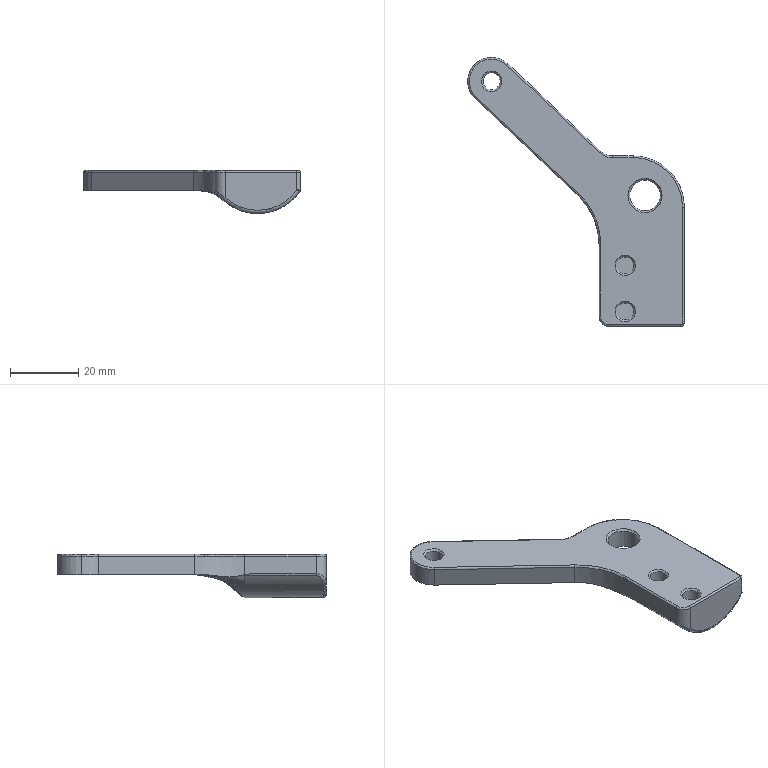Part | STEP file | 101000007782 | 1 solid | 70 faces | box 63.5 x 78.9 x 12.709 mm | volume 13515 mm3 | cylinder 27 | spline 13 | cone 10 | plane 10 | torus 8 | sphere 2 | commonest cylinder face diameters 1 x7 5 x6 2 x2 9 x2 14 x2 20 x2